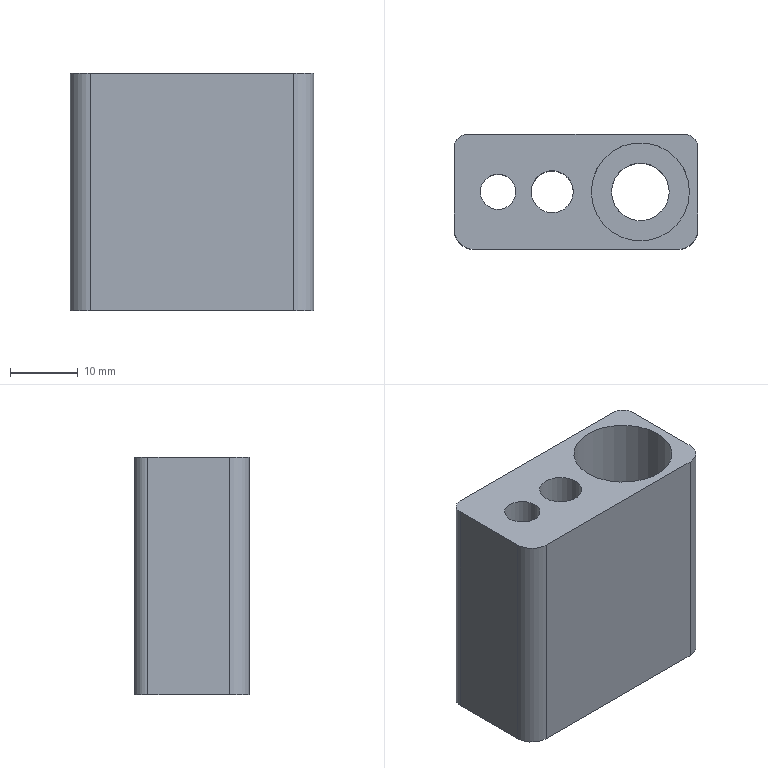Part | NX | features DIE-102 2 | 1 solid | 18 faces | box 36 x 17 x 35 mm | volume 15865 mm3 | cylinder 10 | plane 8 | commonest cylinder face diameters 4 x2 6 x2 5.2 x1 6.2 x1 8.5 x1 9 x1
STEP:
#1=CARTESIAN_POINT('',(4211.836,-839.122,858.716));
#2=VERTEX_POINT('',#1);
#3=CARTESIAN_POINT('',(4209.236,-839.122,858.716));
#4=DIRECTION('',(0.,0.,1.));
#5=DIRECTION('',(1.,0.,0.));
#6=AXIS2_PLACEMENT_3D('',#3,#4,#5);
#7=CIRCLE('',#6,2.6);
#8=EDGE_CURVE('',#2,#2,#7,.F.);
#9=ORIENTED_EDGE('',*,*,#8,.F.);
#10=EDGE_LOOP('',(#9));
#11=FACE_BOUND('',#10,.T.);
#12=CARTESIAN_POINT('',(4206.636,-839.122,828.916));
#13=VERTEX_POINT('',#12);
#14=CARTESIAN_POINT('',(4209.236,-839.122,828.916));
#15=DIRECTION('',(0.,0.,-1.));
#16=DIRECTION('',(-1.,0.,0.));
#17=AXIS2_PLACEMENT_3D('',#14,#15,#16);
#18=CIRCLE('',#17,2.6);
#19=EDGE_CURVE('',#13,#13,#18,.F.);
#20=ORIENTED_EDGE('',*,*,#19,.F.);
#21=EDGE_LOOP('',(#20));
#22=FACE_BOUND('',#21,.T.);
#23=CARTESIAN_POINT('',(4209.236,-839.122,823.716));
#24=DIRECTION('',(0.,0.,1.));
#25=DIRECTION('',(1.,0.,0.));
#26=AXIS2_PLACEMENT_3D('',#23,#24,#25);
#27=CYLINDRICAL_SURFACE('',#26,2.6);
#28=ADVANCED_FACE('',(#11,#22),#27,.F.);
#29=CARTESIAN_POINT('',(4220.336,-839.123,858.716));
#30=VERTEX_POINT('',#29);
#31=CARTESIAN_POINT('',(4217.236,-839.123,858.716));
#32=DIRECTION('',(0.,0.,1.));
#33=DIRECTION('',(1.,0.,0.));
#34=AXIS2_PLACEMENT_3D('',#31,#32,#33);
#35=CIRCLE('',#34,3.1);
#36=EDGE_CURVE('',#30,#30,#35,.F.);
#37=ORIENTED_EDGE('',*,*,#36,.F.);
#38=EDGE_LOOP('',(#37));
#39=FACE_BOUND('',#38,.T.);
#40=CARTESIAN_POINT('',(4214.136,-839.123,828.916));
#41=VERTEX_POINT('',#40);
#42=CARTESIAN_POINT('',(4217.236,-839.123,828.916));
#43=DIRECTION('',(0.,0.,-1.));
#44=DIRECTION('',(-1.,0.,0.));
#45=AXIS2_PLACEMENT_3D('',#42,#43,#44);
#46=CIRCLE('',#45,3.1);
#47=EDGE_CURVE('',#41,#41,#46,.F.);
#48=ORIENTED_EDGE('',*,*,#47,.F.);
#49=EDGE_LOOP('',(#48));
#50=FACE_BOUND('',#49,.T.);
#51=CARTESIAN_POINT('',(4217.236,-839.123,823.716));
#52=DIRECTION('',(0.,0.,1.));
#53=DIRECTION('',(1.,0.,0.));
#54=AXIS2_PLACEMENT_3D('',#51,#52,#53);
#55=CYLINDRICAL_SURFACE('',#54,3.1);
#56=ADVANCED_FACE('',(#39,#50),#55,.F.);
#57=CARTESIAN_POINT('',(4237.486,-839.123,858.716));
#58=VERTEX_POINT('',#57);
#59=CARTESIAN_POINT('',(4230.236,-839.123,858.716));
#60=DIRECTION('',(0.,0.,-1.));
#61=DIRECTION('',(1.,0.,0.));
#62=AXIS2_PLACEMENT_3D('',#59,#60,#61);
#63=CIRCLE('',#62,7.25);
#64=EDGE_CURVE('',#58,#58,#63,.T.);
#65=ORIENTED_EDGE('',*,*,#64,.T.);
#66=EDGE_LOOP('',(#65));
#67=FACE_BOUND('',#66,.T.);
#68=CARTESIAN_POINT('',(4238.736,-832.623,858.716));
#69=VERTEX_POINT('',#68);
#70=CARTESIAN_POINT('',(4238.736,-844.623,858.716));
#71=VERTEX_POINT('',#70);
#72=CARTESIAN_POINT('',(4238.736,-717.123,858.716));
#73=DIRECTION('',(0.,-1.,0.));
#74=VECTOR('',#73,1000.);
#75=LINE('',#72,#74);
#76=EDGE_CURVE('',#69,#71,#75,.T.);
#77=ORIENTED_EDGE('',*,*,#76,.F.);
#78=CARTESIAN_POINT('',(4236.736,-830.623,858.716));
#79=VERTEX_POINT('',#78);
#80=CARTESIAN_POINT('',(4236.736,-832.623,858.716));
#81=DIRECTION('',(0.,0.,-1.));
#82=DIRECTION('',(1.,0.,0.));
#83=AXIS2_PLACEMENT_3D('',#80,#81,#82);
#84=CIRCLE('',#83,2.);
#85=EDGE_CURVE('',#79,#69,#84,.T.);
#86=ORIENTED_EDGE('',*,*,#85,.F.);
#87=CARTESIAN_POINT('',(4204.736,-830.623,858.716));
#88=VERTEX_POINT('',#87);
#89=CARTESIAN_POINT('',(4213.736,-830.623,858.716));
#90=DIRECTION('',(-1.,0.,0.));
#91=VECTOR('',#90,1000.);
#92=LINE('',#89,#91);
#93=EDGE_CURVE('',#79,#88,#92,.T.);
#94=ORIENTED_EDGE('',*,*,#93,.T.);
#95=CARTESIAN_POINT('',(4202.736,-832.623,858.716));
#96=VERTEX_POINT('',#95);
#97=CARTESIAN_POINT('',(4204.736,-832.623,858.716));
#98=DIRECTION('',(0.,0.,-1.));
#99=DIRECTION('',(1.,0.,0.));
#100=AXIS2_PLACEMENT_3D('',#97,#98,#99);
#101=CIRCLE('',#100,2.);
#102=EDGE_CURVE('',#96,#88,#101,.T.);
#103=ORIENTED_EDGE('',*,*,#102,.F.);
#104=CARTESIAN_POINT('',(4202.736,-844.623,858.716));
#105=VERTEX_POINT('',#104);
#106=CARTESIAN_POINT('',(4202.736,-839.123,858.716));
#107=DIRECTION('',(0.,-1.,0.));
#108=VECTOR('',#107,1000.);
#109=LINE('',#106,#108);
#110=EDGE_CURVE('',#96,#105,#109,.T.);
#111=ORIENTED_EDGE('',*,*,#110,.T.);
#112=CARTESIAN_POINT('',(4205.736,-847.623,858.716));
#113=VERTEX_POINT('',#112);
#114=CARTESIAN_POINT('',(4205.736,-844.623,858.716));
#115=DIRECTION('',(0.,0.,-1.));
#116=DIRECTION('',(1.,0.,0.));
#117=AXIS2_PLACEMENT_3D('',#114,#115,#116);
#118=CIRCLE('',#117,3.);
#119=EDGE_CURVE('',#105,#113,#118,.F.);
#120=ORIENTED_EDGE('',*,*,#119,.T.);
#121=CARTESIAN_POINT('',(4235.736,-847.623,858.716));
#122=VERTEX_POINT('',#121);
#123=CARTESIAN_POINT('',(4213.736,-847.623,858.716));
#124=DIRECTION('',(1.,0.,0.));
#125=VECTOR('',#124,1000.);
#126=LINE('',#123,#125);
#127=EDGE_CURVE('',#113,#122,#126,.T.);
#128=ORIENTED_EDGE('',*,*,#127,.T.);
#129=CARTESIAN_POINT('',(4235.736,-844.623,858.716));
#130=DIRECTION('',(0.,0.,-1.));
#131=DIRECTION('',(1.,0.,0.));
#132=AXIS2_PLACEMENT_3D('',#129,#130,#131);
#133=CIRCLE('',#132,3.);
#134=EDGE_CURVE('',#122,#71,#133,.F.);
#135=ORIENTED_EDGE('',*,*,#134,.T.);
#136=EDGE_LOOP('',(#77,#86,#94,#103,#111,#120,#128,#135));
#137=FACE_BOUND('',#136,.T.);
#138=ORIENTED_EDGE('',*,*,#36,.T.);
#139=EDGE_LOOP('',(#138));
#140=FACE_BOUND('',#139,.T.);
#141=ORIENTED_EDGE('',*,*,#8,.T.);
#142=EDGE_LOOP('',(#141));
#143=FACE_BOUND('',#142,.T.);
#144=CARTESIAN_POINT('',(3445.094,-717.123,858.716));
#145=DIRECTION('',(0.,0.,1.));
#146=DIRECTION('',(0.,-1.,0.));
#147=AXIS2_PLACEMENT_3D('',#144,#145,#146);
#148=PLANE('',#147);
#149=ADVANCED_FACE('',(#67,#137,#140,#143),#148,.T.);
#150=ORIENTED_EDGE('',*,*,#19,.T.);
#151=EDGE_LOOP('',(#150));
#152=FACE_BOUND('',#151,.T.);
#153=CARTESIAN_POINT('',(4213.242,-841.195,828.916));
#154=VERTEX_POINT('',#153);
#155=CARTESIAN_POINT('',(4213.242,-837.05,828.916));
#156=VERTEX_POINT('',#155);
#157=CARTESIAN_POINT('',(4209.236,-839.122,828.916));
#158=DIRECTION('',(0.,0.,-1.));
#159=DIRECTION('',(-1.,0.,0.));
#160=AXIS2_PLACEMENT_3D('',#157,#158,#159);
#161=CIRCLE('',#160,4.51);
#162=EDGE_CURVE('',#154,#156,#161,.T.);
#163=ORIENTED_EDGE('',*,*,#162,.T.);
#164=CARTESIAN_POINT('',(4217.236,-839.123,828.916));
#165=DIRECTION('',(0.,0.,1.));
#166=DIRECTION('',(-1.,0.,0.));
#167=AXIS2_PLACEMENT_3D('',#164,#165,#166);
#168=CIRCLE('',#167,4.5);
#169=EDGE_CURVE('',#156,#154,#168,.F.);
#170=ORIENTED_EDGE('',*,*,#169,.T.);
#171=EDGE_LOOP('',(#163,#170));
#172=FACE_BOUND('',#171,.T.);
#173=ORIENTED_EDGE('',*,*,#47,.T.);
#174=EDGE_LOOP('',(#173));
#175=FACE_BOUND('',#174,.T.);
#176=CARTESIAN_POINT('',(4217.236,-839.123,828.916));
#177=DIRECTION('',(0.,0.,-1.));
#178=DIRECTION('',(-1.,0.,0.));
#179=AXIS2_PLACEMENT_3D('',#176,#177,#178);
#180=PLANE('',#179);
#181=ADVANCED_FACE('',(#152,#172,#175),#180,.T.);
#182=CARTESIAN_POINT('',(4213.242,-837.05,823.716));
#183=VERTEX_POINT('',#182);
#184=CARTESIAN_POINT('',(4213.242,-837.05,823.716));
#185=DIRECTION('',(0.,0.,1.));
#186=VECTOR('',#185,1000.);
#187=LINE('',#184,#186);
#188=EDGE_CURVE('',#183,#156,#187,.T.);
#189=ORIENTED_EDGE('',*,*,#188,.T.);
#190=ORIENTED_EDGE('',*,*,#162,.F.);
#191=CARTESIAN_POINT('',(4213.242,-841.195,823.716));
#192=VERTEX_POINT('',#191);
#193=CARTESIAN_POINT('',(4213.242,-841.195,823.716));
#194=DIRECTION('',(0.,0.,-1.));
#195=VECTOR('',#194,1000.);
#196=LINE('',#193,#195);
#197=EDGE_CURVE('',#154,#192,#196,.T.);
#198=ORIENTED_EDGE('',*,*,#197,.T.);
#199=CARTESIAN_POINT('',(4209.236,-839.122,823.716));
#200=DIRECTION('',(0.,0.,1.));
#201=DIRECTION('',(1.,0.,0.));
#202=AXIS2_PLACEMENT_3D('',#199,#200,#201);
#203=CIRCLE('',#202,4.51);
#204=EDGE_CURVE('',#192,#183,#203,.F.);
#205=ORIENTED_EDGE('',*,*,#204,.T.);
#206=EDGE_LOOP('',(#189,#190,#198,#205));
#207=FACE_BOUND('',#206,.T.);
#208=CARTESIAN_POINT('',(4209.236,-839.122,823.716));
#209=DIRECTION('',(0.,0.,1.));
#210=DIRECTION('',(1.,0.,0.));
#211=AXIS2_PLACEMENT_3D('',#208,#209,#210);
#212=CYLINDRICAL_SURFACE('',#211,4.51);
#213=ADVANCED_FACE('',(#207),#212,.F.);
#214=CARTESIAN_POINT('',(4217.236,-839.123,823.716));
#215=DIRECTION('',(0.,0.,-1.));
#216=DIRECTION('',(1.,0.,0.));
#217=AXIS2_PLACEMENT_3D('',#214,#215,#216);
#218=CIRCLE('',#217,4.5);
#219=EDGE_CURVE('',#192,#183,#218,.F.);
#220=ORIENTED_EDGE('',*,*,#219,.F.);
#221=ORIENTED_EDGE('',*,*,#197,.F.);
#222=ORIENTED_EDGE('',*,*,#169,.F.);
#223=ORIENTED_EDGE('',*,*,#188,.F.);
#224=EDGE_LOOP('',(#220,#221,#222,#223));
#225=FACE_BOUND('',#224,.T.);
#226=CARTESIAN_POINT('',(4217.236,-839.123,823.716));
#227=DIRECTION('',(0.,0.,1.));
#228=DIRECTION('',(1.,0.,0.));
#229=AXIS2_PLACEMENT_3D('',#226,#227,#228);
#230=CYLINDRICAL_SURFACE('',#229,4.5);
#231=ADVANCED_FACE('',(#225),#230,.F.);
#232=CARTESIAN_POINT('',(4234.486,-839.123,823.716));
#233=VERTEX_POINT('',#232);
#234=CARTESIAN_POINT('',(4230.236,-839.123,823.716));
#235=DIRECTION('',(0.,0.,-1.));
#236=DIRECTION('',(1.,0.,0.));
#237=AXIS2_PLACEMENT_3D('',#234,#235,#236);
#238=CIRCLE('',#237,4.25);
#239=EDGE_CURVE('',#233,#233,#238,.F.);
#240=ORIENTED_EDGE('',*,*,#239,.T.);
#241=EDGE_LOOP('',(#240));
#242=FACE_BOUND('',#241,.T.);
#243=CARTESIAN_POINT('',(4235.736,-847.623,823.716));
#244=VERTEX_POINT('',#243);
#245=CARTESIAN_POINT('',(4205.736,-847.623,823.716));
#246=VERTEX_POINT('',#245);
#247=CARTESIAN_POINT('',(4213.736,-847.623,823.716));
#248=DIRECTION('',(1.,0.,0.));
#249=VECTOR('',#248,1000.);
#250=LINE('',#247,#249);
#251=EDGE_CURVE('',#244,#246,#250,.F.);
#252=ORIENTED_EDGE('',*,*,#251,.T.);
#253=CARTESIAN_POINT('',(4202.736,-844.623,823.716));
#254=VERTEX_POINT('',#253);
#255=CARTESIAN_POINT('',(4205.736,-844.623,823.716));
#256=DIRECTION('',(0.,0.,1.));
#257=DIRECTION('',(-1.,0.,0.));
#258=AXIS2_PLACEMENT_3D('',#255,#256,#257);
#259=CIRCLE('',#258,3.);
#260=EDGE_CURVE('',#254,#246,#259,.T.);
#261=ORIENTED_EDGE('',*,*,#260,.F.);
#262=CARTESIAN_POINT('',(4202.736,-832.623,823.716));
#263=VERTEX_POINT('',#262);
#264=CARTESIAN_POINT('',(4202.736,-839.123,823.716));
#265=DIRECTION('',(0.,1.,0.));
#266=VECTOR('',#265,1000.);
#267=LINE('',#264,#266);
#268=EDGE_CURVE('',#254,#263,#267,.T.);
#269=ORIENTED_EDGE('',*,*,#268,.T.);
#270=CARTESIAN_POINT('',(4204.736,-830.623,823.716));
#271=VERTEX_POINT('',#270);
#272=CARTESIAN_POINT('',(4204.736,-832.623,823.716));
#273=DIRECTION('',(0.,0.,1.));
#274=DIRECTION('',(-1.,0.,0.));
#275=AXIS2_PLACEMENT_3D('',#272,#273,#274);
#276=CIRCLE('',#275,2.);
#277=EDGE_CURVE('',#271,#263,#276,.T.);
#278=ORIENTED_EDGE('',*,*,#277,.F.);
#279=CARTESIAN_POINT('',(4236.736,-830.623,823.716));
#280=VERTEX_POINT('',#279);
#281=CARTESIAN_POINT('',(4213.736,-830.623,823.716));
#282=DIRECTION('',(-1.,0.,0.));
#283=VECTOR('',#282,1000.);
#284=LINE('',#281,#283);
#285=EDGE_CURVE('',#271,#280,#284,.F.);
#286=ORIENTED_EDGE('',*,*,#285,.T.);
#287=CARTESIAN_POINT('',(4238.736,-832.623,823.716));
#288=VERTEX_POINT('',#287);
#289=CARTESIAN_POINT('',(4236.736,-832.623,823.716));
#290=DIRECTION('',(0.,0.,1.));
#291=DIRECTION('',(-1.,0.,0.));
#292=AXIS2_PLACEMENT_3D('',#289,#290,#291);
#293=CIRCLE('',#292,2.);
#294=EDGE_CURVE('',#288,#280,#293,.T.);
#295=ORIENTED_EDGE('',*,*,#294,.F.);
#296=CARTESIAN_POINT('',(4238.736,-844.623,823.716));
#297=VERTEX_POINT('',#296);
#298=CARTESIAN_POINT('',(4238.736,-839.123,823.716));
#299=DIRECTION('',(0.,1.,0.));
#300=VECTOR('',#299,1000.);
#301=LINE('',#298,#300);
#302=EDGE_CURVE('',#288,#297,#301,.F.);
#303=ORIENTED_EDGE('',*,*,#302,.T.);
#304=CARTESIAN_POINT('',(4235.736,-844.623,823.716));
#305=DIRECTION('',(0.,0.,1.));
#306=DIRECTION('',(-1.,0.,0.));
#307=AXIS2_PLACEMENT_3D('',#304,#305,#306);
#308=CIRCLE('',#307,3.);
#309=EDGE_CURVE('',#297,#244,#308,.F.);
#310=ORIENTED_EDGE('',*,*,#309,.T.);
#311=EDGE_LOOP('',(#252,#261,#269,#278,#286,#295,#303,#310));
#312=FACE_BOUND('',#311,.T.);
#313=ORIENTED_EDGE('',*,*,#219,.T.);
#314=ORIENTED_EDGE('',*,*,#204,.F.);
#315=EDGE_LOOP('',(#313,#314));
#316=FACE_BOUND('',#315,.T.);
#317=CARTESIAN_POINT('',(3445.094,-717.123,823.716));
#318=DIRECTION('',(0.,0.,1.));
#319=DIRECTION('',(0.,-1.,0.));
#320=AXIS2_PLACEMENT_3D('',#317,#318,#319);
#321=PLANE('',#320);
#322=ADVANCED_FACE('',(#242,#312,#316),#321,.F.);
#323=ORIENTED_EDGE('',*,*,#285,.F.);
#324=CARTESIAN_POINT('',(4204.736,-830.623,828.716));
#325=DIRECTION('',(0.,0.,1.));
#326=VECTOR('',#325,1000.);
#327=LINE('',#324,#326);
#328=EDGE_CURVE('',#88,#271,#327,.F.);
#329=ORIENTED_EDGE('',*,*,#328,.F.);
#330=ORIENTED_EDGE('',*,*,#93,.F.);
#331=CARTESIAN_POINT('',(4236.736,-830.623,828.716));
#332=DIRECTION('',(0.,0.,1.));
#333=VECTOR('',#332,1000.);
#334=LINE('',#331,#333);
#335=EDGE_CURVE('',#280,#79,#334,.T.);
#336=ORIENTED_EDGE('',*,*,#335,.F.);
#337=EDGE_LOOP('',(#323,#329,#330,#336));
#338=FACE_BOUND('',#337,.T.);
#339=CARTESIAN_POINT('',(4213.736,-830.623,828.716));
#340=DIRECTION('',(0.,1.,0.));
#341=DIRECTION('',(0.,0.,-1.));
#342=AXIS2_PLACEMENT_3D('',#339,#340,#341);
#343=PLANE('',#342);
#344=ADVANCED_FACE('',(#338),#343,.T.);
#345=ORIENTED_EDGE('',*,*,#268,.F.);
#346=CARTESIAN_POINT('',(4202.736,-844.623,828.716));
#347=DIRECTION('',(0.,0.,1.));
#348=VECTOR('',#347,1000.);
#349=LINE('',#346,#348);
#350=EDGE_CURVE('',#105,#254,#349,.F.);
#351=ORIENTED_EDGE('',*,*,#350,.F.);
#352=ORIENTED_EDGE('',*,*,#110,.F.);
#353=CARTESIAN_POINT('',(4202.736,-832.623,828.716));
#354=DIRECTION('',(0.,0.,1.));
#355=VECTOR('',#354,1000.);
#356=LINE('',#353,#355);
#357=EDGE_CURVE('',#263,#96,#356,.T.);
#358=ORIENTED_EDGE('',*,*,#357,.F.);
#359=EDGE_LOOP('',(#345,#351,#352,#358));
#360=FACE_BOUND('',#359,.T.);
#361=CARTESIAN_POINT('',(4202.736,-839.123,828.716));
#362=DIRECTION('',(-1.,0.,0.));
#363=DIRECTION('',(0.,0.,1.));
#364=AXIS2_PLACEMENT_3D('',#361,#362,#363);
#365=PLANE('',#364);
#366=ADVANCED_FACE('',(#360),#365,.T.);
#367=ORIENTED_EDGE('',*,*,#127,.F.);
#368=CARTESIAN_POINT('',(4205.736,-847.623,828.716));
#369=DIRECTION('',(0.,0.,1.));
#370=VECTOR('',#369,1000.);
#371=LINE('',#368,#370);
#372=EDGE_CURVE('',#246,#113,#371,.T.);
#373=ORIENTED_EDGE('',*,*,#372,.F.);
#374=ORIENTED_EDGE('',*,*,#251,.F.);
#375=CARTESIAN_POINT('',(4235.736,-847.623,828.716));
#376=DIRECTION('',(0.,0.,1.));
#377=VECTOR('',#376,1000.);
#378=LINE('',#375,#377);
#379=EDGE_CURVE('',#122,#244,#378,.F.);
#380=ORIENTED_EDGE('',*,*,#379,.F.);
#381=EDGE_LOOP('',(#367,#373,#374,#380));
#382=FACE_BOUND('',#381,.T.);
#383=CARTESIAN_POINT('',(4213.736,-847.623,828.716));
#384=DIRECTION('',(0.,-1.,0.));
#385=DIRECTION('',(0.,0.,1.));
#386=AXIS2_PLACEMENT_3D('',#383,#384,#385);
#387=PLANE('',#386);
#388=ADVANCED_FACE('',(#382),#387,.T.);
#389=ORIENTED_EDGE('',*,*,#76,.T.);
#390=CARTESIAN_POINT('',(4238.736,-844.623,828.716));
#391=DIRECTION('',(0.,0.,1.));
#392=VECTOR('',#391,1000.);
#393=LINE('',#390,#392);
#394=EDGE_CURVE('',#297,#71,#393,.T.);
#395=ORIENTED_EDGE('',*,*,#394,.F.);
#396=ORIENTED_EDGE('',*,*,#302,.F.);
#397=CARTESIAN_POINT('',(4238.736,-832.623,828.716));
#398=DIRECTION('',(0.,0.,1.));
#399=VECTOR('',#398,1000.);
#400=LINE('',#397,#399);
#401=EDGE_CURVE('',#69,#288,#400,.F.);
#402=ORIENTED_EDGE('',*,*,#401,.F.);
#403=EDGE_LOOP('',(#389,#395,#396,#402));
#404=FACE_BOUND('',#403,.T.);
#405=CARTESIAN_POINT('',(4238.736,-839.123,828.716));
#406=DIRECTION('',(1.,0.,0.));
#407=DIRECTION('',(0.,0.,-1.));
#408=AXIS2_PLACEMENT_3D('',#405,#406,#407);
#409=PLANE('',#408);
#410=ADVANCED_FACE('',(#404),#409,.T.);
#411=ORIENTED_EDGE('',*,*,#309,.F.);
#412=ORIENTED_EDGE('',*,*,#394,.T.);
#413=ORIENTED_EDGE('',*,*,#134,.F.);
#414=ORIENTED_EDGE('',*,*,#379,.T.);
#415=EDGE_LOOP('',(#411,#412,#413,#414));
#416=FACE_BOUND('',#415,.T.);
#417=CARTESIAN_POINT('',(4235.736,-844.623,828.716));
#418=DIRECTION('',(0.,0.,1.));
#419=DIRECTION('',(1.,0.,0.));
#420=AXIS2_PLACEMENT_3D('',#417,#418,#419);
#421=CYLINDRICAL_SURFACE('',#420,3.);
#422=ADVANCED_FACE('',(#416),#421,.T.);
#423=ORIENTED_EDGE('',*,*,#260,.T.);
#424=ORIENTED_EDGE('',*,*,#372,.T.);
#425=ORIENTED_EDGE('',*,*,#119,.F.);
#426=ORIENTED_EDGE('',*,*,#350,.T.);
#427=EDGE_LOOP('',(#423,#424,#425,#426));
#428=FACE_BOUND('',#427,.T.);
#429=CARTESIAN_POINT('',(4205.736,-844.623,828.716));
#430=DIRECTION('',(0.,0.,1.));
#431=DIRECTION('',(1.,0.,0.));
#432=AXIS2_PLACEMENT_3D('',#429,#430,#431);
#433=CYLINDRICAL_SURFACE('',#432,3.);
#434=ADVANCED_FACE('',(#428),#433,.T.);
#435=ORIENTED_EDGE('',*,*,#294,.T.);
#436=ORIENTED_EDGE('',*,*,#335,.T.);
#437=ORIENTED_EDGE('',*,*,#85,.T.);
#438=ORIENTED_EDGE('',*,*,#401,.T.);
#439=EDGE_LOOP('',(#435,#436,#437,#438));
#440=FACE_BOUND('',#439,.T.);
#441=CARTESIAN_POINT('',(4236.736,-832.623,828.716));
#442=DIRECTION('',(0.,0.,1.));
#443=DIRECTION('',(1.,0.,0.));
#444=AXIS2_PLACEMENT_3D('',#441,#442,#443);
#445=CYLINDRICAL_SURFACE('',#444,2.);
#446=ADVANCED_FACE('',(#440),#445,.T.);
#447=ORIENTED_EDGE('',*,*,#277,.T.);
#448=ORIENTED_EDGE('',*,*,#357,.T.);
#449=ORIENTED_EDGE('',*,*,#102,.T.);
#450=ORIENTED_EDGE('',*,*,#328,.T.);
#451=EDGE_LOOP('',(#447,#448,#449,#450));
#452=FACE_BOUND('',#451,.T.);
#453=CARTESIAN_POINT('',(4204.736,-832.623,828.716));
#454=DIRECTION('',(0.,0.,1.));
#455=DIRECTION('',(1.,0.,0.));
#456=AXIS2_PLACEMENT_3D('',#453,#454,#455);
#457=CYLINDRICAL_SURFACE('',#456,2.);
#458=ADVANCED_FACE('',(#452),#457,.T.);
#459=ORIENTED_EDGE('',*,*,#239,.F.);
#460=EDGE_LOOP('',(#459));
#461=FACE_BOUND('',#460,.T.);
#462=CARTESIAN_POINT('',(4234.486,-839.123,847.716));
#463=VERTEX_POINT('',#462);
#464=CARTESIAN_POINT('',(4230.236,-839.123,847.716));
#465=DIRECTION('',(0.,0.,-1.));
#466=DIRECTION('',(1.,0.,0.));
#467=AXIS2_PLACEMENT_3D('',#464,#465,#466);
#468=CIRCLE('',#467,4.25);
#469=EDGE_CURVE('',#463,#463,#468,.T.);
#470=ORIENTED_EDGE('',*,*,#469,.F.);
#471=EDGE_LOOP('',(#470));
#472=FACE_BOUND('',#471,.T.);
#473=CARTESIAN_POINT('',(4230.236,-839.123,822.716));
#474=DIRECTION('',(0.,0.,1.));
#475=DIRECTION('',(1.,0.,0.));
#476=AXIS2_PLACEMENT_3D('',#473,#474,#475);
#477=CYLINDRICAL_SURFACE('',#476,4.25);
#478=ADVANCED_FACE('',(#461,#472),#477,.F.);
#479=ORIENTED_EDGE('',*,*,#64,.F.);
#480=EDGE_LOOP('',(#479));
#481=FACE_BOUND('',#480,.T.);
#482=CARTESIAN_POINT('',(4237.486,-839.123,847.716));
#483=VERTEX_POINT('',#482);
#484=CARTESIAN_POINT('',(4230.236,-839.123,847.716));
#485=DIRECTION('',(0.,0.,-1.));
#486=DIRECTION('',(1.,0.,0.));
#487=AXIS2_PLACEMENT_3D('',#484,#485,#486);
#488=CIRCLE('',#487,7.25);
#489=EDGE_CURVE('',#483,#483,#488,.F.);
#490=ORIENTED_EDGE('',*,*,#489,.F.);
#491=EDGE_LOOP('',(#490));
#492=FACE_BOUND('',#491,.T.);
#493=CARTESIAN_POINT('',(4230.236,-839.123,847.716));
#494=DIRECTION('',(0.,0.,1.));
#495=DIRECTION('',(1.,0.,0.));
#496=AXIS2_PLACEMENT_3D('',#493,#494,#495);
#497=CYLINDRICAL_SURFACE('',#496,7.25);
#498=ADVANCED_FACE('',(#481,#492),#497,.F.);
#499=ORIENTED_EDGE('',*,*,#469,.T.);
#500=EDGE_LOOP('',(#499));
#501=FACE_BOUND('',#500,.T.);
#502=ORIENTED_EDGE('',*,*,#489,.T.);
#503=EDGE_LOOP('',(#502));
#504=FACE_BOUND('',#503,.T.);
#505=CARTESIAN_POINT('',(4230.236,-839.123,847.716));
#506=DIRECTION('',(0.,0.,1.));
#507=DIRECTION('',(1.,0.,0.));
#508=AXIS2_PLACEMENT_3D('',#505,#506,#507);
#509=PLANE('',#508);
#510=ADVANCED_FACE('',(#501,#504),#509,.T.);
#511=CLOSED_SHELL('',(#28,#56,#149,#181,#213,#231,#322,#344,#366,#388,#410,#422,#434,#446,#458,#478,#498,#510));
#512=MANIFOLD_SOLID_BREP('',#511);
#513=(LENGTH_UNIT()NAMED_UNIT(*)SI_UNIT(.MILLI.,.METRE.));
#514=UNCERTAINTY_MEASURE_WITH_UNIT(LENGTH_MEASURE(0.00001),#513,'','');
#515=(NAMED_UNIT(*)PLANE_ANGLE_UNIT()SI_UNIT($,.RADIAN.));
#516=(NAMED_UNIT(*)SI_UNIT($,.STERADIAN.)SOLID_ANGLE_UNIT());
#517=(GEOMETRIC_REPRESENTATION_CONTEXT(3)GLOBAL_UNCERTAINTY_ASSIGNED_CONTEXT((#514))GLOBAL_UNIT_ASSIGNED_CONTEXT((#513,#515,#516))REPRESENTATION_CONTEXT('',''));
#518=ADVANCED_BREP_SHAPE_REPRESENTATION('',(#512),#517);